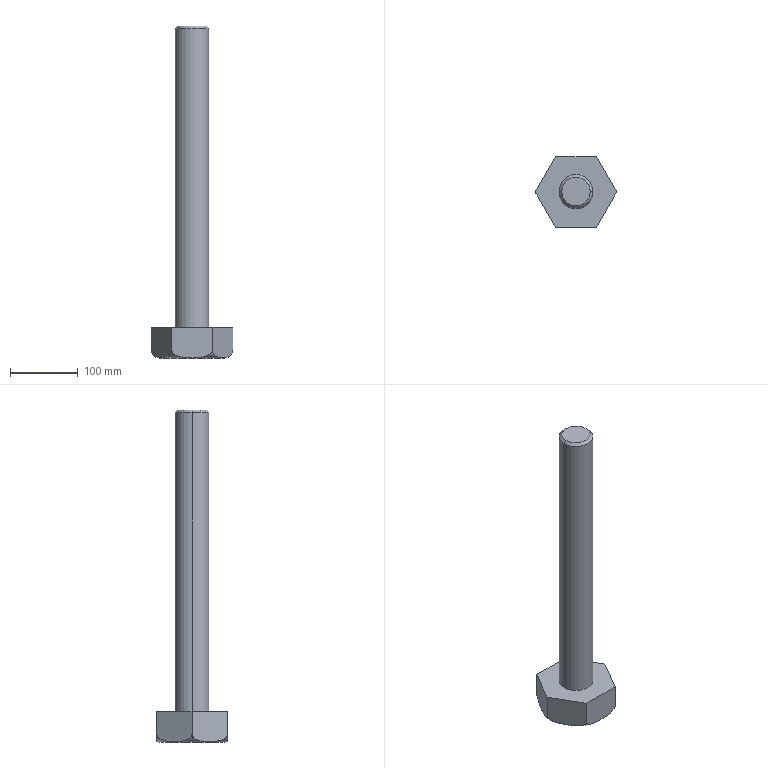Part | SolidWorks | features Chamfer 1, Extrusion 1, ICE 1, RevCut 1 | 1 solid | 15 faces | box 120.089 x 104 x 490 mm | volume 1291940 mm3 | plane 9 | cone 2 | cylinder 2 | torus 2 | commonest cylinder face diameters 50 x2
STEP:
#1=CARTESIAN_POINT('',(21.,0.,490.));
#2=VERTEX_POINT('',#1);
#3=CARTESIAN_POINT('',(-21.,0.,490.));
#4=VERTEX_POINT('',#3);
#5=CARTESIAN_POINT('',(0.,0.,490.));
#6=DIRECTION('',(0.,0.,1.));
#7=DIRECTION('',(1.,0.,0.));
#8=AXIS2_PLACEMENT_3D('',#5,#6,#7);
#9=CIRCLE('',#8,21.);
#10=EDGE_CURVE('',#2,#4,#9,.T.);
#11=ORIENTED_EDGE('',*,*,#10,.F.);
#12=CARTESIAN_POINT('',(25.,0.,486.));
#13=VERTEX_POINT('',#12);
#14=CARTESIAN_POINT('',(21.,0.,490.));
#15=DIRECTION('',(0.7071,0.,-0.7071));
#16=VECTOR('',#15,1000.);
#17=LINE('',#14,#16);
#18=EDGE_CURVE('',#2,#13,#17,.T.);
#19=ORIENTED_EDGE('',*,*,#18,.T.);
#20=CARTESIAN_POINT('',(-25.,0.,486.));
#21=VERTEX_POINT('',#20);
#22=CARTESIAN_POINT('',(0.,0.,486.));
#23=DIRECTION('',(0.,0.,-1.));
#24=DIRECTION('',(1.,0.,0.));
#25=AXIS2_PLACEMENT_3D('',#22,#23,#24);
#26=CIRCLE('',#25,25.);
#27=EDGE_CURVE('',#21,#13,#26,.T.);
#28=ORIENTED_EDGE('',*,*,#27,.F.);
#29=CARTESIAN_POINT('',(-21.,0.,490.));
#30=DIRECTION('',(-0.7071,0.,-0.7071));
#31=VECTOR('',#30,1000.);
#32=LINE('',#29,#31);
#33=EDGE_CURVE('',#4,#21,#32,.T.);
#34=ORIENTED_EDGE('',*,*,#33,.F.);
#35=EDGE_LOOP('',(#11,#19,#28,#34));
#36=FACE_OUTER_BOUND('',#35,.T.);
#37=CARTESIAN_POINT('',(0.,0.,490.));
#38=DIRECTION('',(0.,0.,-1.));
#39=DIRECTION('',(-1.,0.,0.));
#40=AXIS2_PLACEMENT_3D('',#37,#38,#39);
#41=CONICAL_SURFACE('',#40,21.,0.7854);
#42=ADVANCED_FACE('',(#36),#41,.T.);
#43=ORIENTED_EDGE('',*,*,#27,.T.);
#44=CARTESIAN_POINT('',(25.,0.,45.));
#45=VERTEX_POINT('',#44);
#46=CARTESIAN_POINT('',(25.,0.,490.));
#47=DIRECTION('',(0.,0.,-1.));
#48=VECTOR('',#47,1000.);
#49=LINE('',#46,#48);
#50=EDGE_CURVE('',#13,#45,#49,.T.);
#51=ORIENTED_EDGE('',*,*,#50,.T.);
#52=CARTESIAN_POINT('',(-25.,0.,45.));
#53=VERTEX_POINT('',#52);
#54=CARTESIAN_POINT('',(0.,0.,45.));
#55=DIRECTION('',(0.,0.,1.));
#56=DIRECTION('',(1.,0.,0.));
#57=AXIS2_PLACEMENT_3D('',#54,#55,#56);
#58=CIRCLE('',#57,25.);
#59=EDGE_CURVE('',#45,#53,#58,.T.);
#60=ORIENTED_EDGE('',*,*,#59,.T.);
#61=CARTESIAN_POINT('',(-25.,0.,490.));
#62=DIRECTION('',(0.,0.,-1.));
#63=VECTOR('',#62,1000.);
#64=LINE('',#61,#63);
#65=EDGE_CURVE('',#21,#53,#64,.T.);
#66=ORIENTED_EDGE('',*,*,#65,.F.);
#67=EDGE_LOOP('',(#43,#51,#60,#66));
#68=FACE_OUTER_BOUND('',#67,.T.);
#69=CARTESIAN_POINT('',(0.,0.,490.));
#70=DIRECTION('',(0.,0.,-1.));
#71=DIRECTION('',(-1.,0.,0.));
#72=AXIS2_PLACEMENT_3D('',#69,#70,#71);
#73=CYLINDRICAL_SURFACE('',#72,25.);
#74=ADVANCED_FACE('',(#68),#73,.T.);
#75=CARTESIAN_POINT('',(60.044,0.,12.));
#76=VERTEX_POINT('',#75);
#77=CARTESIAN_POINT('',(30.022,52.,12.));
#78=VERTEX_POINT('',#77);
#79=CARTESIAN_POINT('',(60.044,0.,12.));
#80=CARTESIAN_POINT('',(60.044,0.,11.26));
#81=CARTESIAN_POINT('',(59.977,0.1174,10.543));
#82=CARTESIAN_POINT('',(59.786,0.4482,9.504));
#83=CARTESIAN_POINT('',(59.709,0.5818,9.172));
#84=CARTESIAN_POINT('',(59.531,0.8892,8.533));
#85=CARTESIAN_POINT('',(59.43,1.064,8.225));
#86=CARTESIAN_POINT('',(59.1,1.636,7.342));
#87=CARTESIAN_POINT('',(58.847,2.074,6.819));
#88=CARTESIAN_POINT('',(58.296,3.028,5.867));
#89=CARTESIAN_POINT('',(57.996,3.549,5.437));
#90=CARTESIAN_POINT('',(57.376,4.621,4.673));
#91=CARTESIAN_POINT('',(57.056,5.177,4.336));
#92=CARTESIAN_POINT('',(56.398,6.316,3.728));
#93=CARTESIAN_POINT('',(56.061,6.9,3.458));
#94=CARTESIAN_POINT('',(55.373,8.092,2.971));
#95=CARTESIAN_POINT('',(55.024,8.695,2.757));
#96=CARTESIAN_POINT('',(54.326,9.905,2.375));
#97=CARTESIAN_POINT('',(53.975,10.513,2.207));
#98=CARTESIAN_POINT('',(52.919,12.342,1.759));
#99=CARTESIAN_POINT('',(52.209,13.571,1.533));
#100=CARTESIAN_POINT('',(50.783,16.041,1.175));
#101=CARTESIAN_POINT('',(50.066,17.282,1.044));
#102=CARTESIAN_POINT('',(48.629,19.773,0.8452));
#103=CARTESIAN_POINT('',(47.907,21.022,0.778));
#104=CARTESIAN_POINT('',(46.462,23.525,0.6906));
#105=CARTESIAN_POINT('',(45.74,24.776,0.6704));
#106=CARTESIAN_POINT('',(44.296,27.278,0.671));
#107=CARTESIAN_POINT('',(43.573,28.529,0.6918));
#108=CARTESIAN_POINT('',(42.129,31.03,0.7805));
#109=CARTESIAN_POINT('',(41.407,32.281,0.8485));
#110=CARTESIAN_POINT('',(39.966,34.777,1.05));
#111=CARTESIAN_POINT('',(39.248,36.021,1.183));
#112=CARTESIAN_POINT('',(37.817,38.5,1.545));
#113=CARTESIAN_POINT('',(37.104,39.735,1.775));
#114=CARTESIAN_POINT('',(35.687,42.188,2.382));
#115=CARTESIAN_POINT('',(34.991,43.394,2.757));
#116=CARTESIAN_POINT('',(33.974,45.156,3.483));
#117=CARTESIAN_POINT('',(33.639,45.735,3.753));
#118=CARTESIAN_POINT('',(32.982,46.873,4.365));
#119=CARTESIAN_POINT('',(32.66,47.431,4.707));
#120=CARTESIAN_POINT('',(32.046,48.494,5.471));
#121=CARTESIAN_POINT('',(31.753,49.002,5.893));
#122=CARTESIAN_POINT('',(31.203,49.954,6.85));
#123=CARTESIAN_POINT('',(30.953,50.387,7.374));
#124=CARTESIAN_POINT('',(30.63,50.948,8.245));
#125=CARTESIAN_POINT('',(30.53,51.12,8.551));
#126=CARTESIAN_POINT('',(30.354,51.426,9.19));
#127=CARTESIAN_POINT('',(30.278,51.557,9.519));
#128=CARTESIAN_POINT('',(30.154,51.772,10.198));
#129=CARTESIAN_POINT('',(30.105,51.857,10.55));
#130=CARTESIAN_POINT('',(30.039,51.971,11.27));
#131=CARTESIAN_POINT('',(30.022,52.,11.633));
#132=CARTESIAN_POINT('',(30.022,52.,12.));
#133=B_SPLINE_CURVE_WITH_KNOTS('',3,(#79,#80,#81,#82,#83,#84,#85,#86,#87,#88,#89,#90,#91,#92,#93,#94,#95,#96,#97,#98,#99,#100,#101,#102,#103,#104,#105,#106,#107,#108,#109,#110,#111,#112,#113,#114,#115,#116,#117,#118,#119,#120,#121,#122,#123,#124,#125,#126,#127,#128,#129,#130,#131,#132),.UNSPECIFIED.,.F.,.F.,(4,2,2,2,2,2,2,2,2,2,2,2,2,2,2,2,2,2,2,2,2,2,2,2,2,2,4),(0.000000197,0.002185,0.003278,0.00437,0.006555,0.00874,0.01093,0.01311,0.0153,0.01748,0.02185,0.02622,0.03059,0.03496,0.03933,0.0437,0.04807,0.05244,0.05681,0.059,0.06118,0.06337,0.06555,0.06664,0.06774,0.06883,0.06992),.UNSPECIFIED.);
#134=EDGE_CURVE('',#76,#78,#133,.T.);
#135=ORIENTED_EDGE('',*,*,#134,.F.);
#136=CARTESIAN_POINT('',(48.044,0.,0.));
#137=VERTEX_POINT('',#136);
#138=CARTESIAN_POINT('',(48.044,0.,12.));
#139=DIRECTION('',(0.,1.,0.));
#140=DIRECTION('',(-1.,0.,0.));
#141=AXIS2_PLACEMENT_3D('',#138,#139,#140);
#142=CIRCLE('',#141,12.);
#143=EDGE_CURVE('',#76,#137,#142,.T.);
#144=ORIENTED_EDGE('',*,*,#143,.T.);
#145=CARTESIAN_POINT('',(-48.044,0.,0.));
#146=VERTEX_POINT('',#145);
#147=CARTESIAN_POINT('',(0.,0.,0.));
#148=DIRECTION('',(0.,0.,-1.));
#149=DIRECTION('',(-1.,0.,0.));
#150=AXIS2_PLACEMENT_3D('',#147,#148,#149);
#151=CIRCLE('',#150,48.044);
#152=EDGE_CURVE('',#146,#137,#151,.T.);
#153=ORIENTED_EDGE('',*,*,#152,.F.);
#154=CARTESIAN_POINT('',(-60.044,0.,12.));
#155=VERTEX_POINT('',#154);
#156=CARTESIAN_POINT('',(-48.044,0.,12.));
#157=DIRECTION('',(0.,-1.,0.));
#158=DIRECTION('',(0.,0.,-1.));
#159=AXIS2_PLACEMENT_3D('',#156,#157,#158);
#160=CIRCLE('',#159,12.);
#161=EDGE_CURVE('',#155,#146,#160,.T.);
#162=ORIENTED_EDGE('',*,*,#161,.F.);
#163=CARTESIAN_POINT('',(-30.022,52.,12.));
#164=VERTEX_POINT('',#163);
#165=CARTESIAN_POINT('',(-30.022,52.,12.));
#166=CARTESIAN_POINT('',(-30.022,52.,11.26));
#167=CARTESIAN_POINT('',(-30.09,51.883,10.543));
#168=CARTESIAN_POINT('',(-30.281,51.552,9.504));
#169=CARTESIAN_POINT('',(-30.358,51.418,9.172));
#170=CARTESIAN_POINT('',(-30.536,51.111,8.533));
#171=CARTESIAN_POINT('',(-30.636,50.936,8.225));
#172=CARTESIAN_POINT('',(-30.967,50.364,7.342));
#173=CARTESIAN_POINT('',(-31.22,49.926,6.819));
#174=CARTESIAN_POINT('',(-31.77,48.972,5.867));
#175=CARTESIAN_POINT('',(-32.071,48.451,5.437));
#176=CARTESIAN_POINT('',(-32.69,47.379,4.673));
#177=CARTESIAN_POINT('',(-33.011,46.823,4.336));
#178=CARTESIAN_POINT('',(-33.669,45.684,3.728));
#179=CARTESIAN_POINT('',(-34.006,45.1,3.458));
#180=CARTESIAN_POINT('',(-34.694,43.908,2.971));
#181=CARTESIAN_POINT('',(-35.043,43.305,2.757));
#182=CARTESIAN_POINT('',(-35.741,42.095,2.375));
#183=CARTESIAN_POINT('',(-36.092,41.487,2.207));
#184=CARTESIAN_POINT('',(-37.148,39.658,1.759));
#185=CARTESIAN_POINT('',(-37.858,38.429,1.533));
#186=CARTESIAN_POINT('',(-39.284,35.959,1.175));
#187=CARTESIAN_POINT('',(-40.,34.718,1.044));
#188=CARTESIAN_POINT('',(-41.438,32.227,0.8452));
#189=CARTESIAN_POINT('',(-42.159,30.978,0.778));
#190=CARTESIAN_POINT('',(-43.604,28.475,0.6906));
#191=CARTESIAN_POINT('',(-44.327,27.224,0.6704));
#192=CARTESIAN_POINT('',(-45.771,24.722,0.671));
#193=CARTESIAN_POINT('',(-46.493,23.471,0.6918));
#194=CARTESIAN_POINT('',(-47.937,20.97,0.7805));
#195=CARTESIAN_POINT('',(-48.66,19.719,0.8485));
#196=CARTESIAN_POINT('',(-50.101,17.223,1.05));
#197=CARTESIAN_POINT('',(-50.819,15.979,1.183));
#198=CARTESIAN_POINT('',(-52.25,13.5,1.545));
#199=CARTESIAN_POINT('',(-52.963,12.265,1.775));
#200=CARTESIAN_POINT('',(-54.38,9.812,2.382));
#201=CARTESIAN_POINT('',(-55.076,8.606,2.757));
#202=CARTESIAN_POINT('',(-56.093,6.844,3.483));
#203=CARTESIAN_POINT('',(-56.427,6.265,3.753));
#204=CARTESIAN_POINT('',(-57.084,5.127,4.365));
#205=CARTESIAN_POINT('',(-57.406,4.569,4.707));
#206=CARTESIAN_POINT('',(-58.02,3.506,5.471));
#207=CARTESIAN_POINT('',(-58.314,2.998,5.893));
#208=CARTESIAN_POINT('',(-58.863,2.046,6.85));
#209=CARTESIAN_POINT('',(-59.113,1.613,7.374));
#210=CARTESIAN_POINT('',(-59.437,1.052,8.245));
#211=CARTESIAN_POINT('',(-59.537,0.8795,8.551));
#212=CARTESIAN_POINT('',(-59.713,0.5743,9.19));
#213=CARTESIAN_POINT('',(-59.789,0.4431,9.519));
#214=CARTESIAN_POINT('',(-59.913,0.2276,10.198));
#215=CARTESIAN_POINT('',(-59.962,0.1431,10.55));
#216=CARTESIAN_POINT('',(-60.028,0.02903,11.27));
#217=CARTESIAN_POINT('',(-60.044,0.,11.633));
#218=CARTESIAN_POINT('',(-60.044,0.,12.));
#219=B_SPLINE_CURVE_WITH_KNOTS('',3,(#165,#166,#167,#168,#169,#170,#171,#172,#173,#174,#175,#176,#177,#178,#179,#180,#181,#182,#183,#184,#185,#186,#187,#188,#189,#190,#191,#192,#193,#194,#195,#196,#197,#198,#199,#200,#201,#202,#203,#204,#205,#206,#207,#208,#209,#210,#211,#212,#213,#214,#215,#216,#217,#218),.UNSPECIFIED.,.F.,.F.,(4,2,2,2,2,2,2,2,2,2,2,2,2,2,2,2,2,2,2,2,2,2,2,2,2,2,4),(0.000000197,0.002185,0.003278,0.00437,0.006555,0.00874,0.01093,0.01311,0.0153,0.01748,0.02185,0.02622,0.03059,0.03496,0.03933,0.0437,0.04807,0.05244,0.05681,0.059,0.06118,0.06337,0.06555,0.06664,0.06774,0.06883,0.06992),.UNSPECIFIED.);
#220=EDGE_CURVE('',#164,#155,#219,.T.);
#221=ORIENTED_EDGE('',*,*,#220,.F.);
#222=CARTESIAN_POINT('',(30.022,52.,12.));
#223=CARTESIAN_POINT('',(30.022,52.,11.638));
#224=CARTESIAN_POINT('',(29.99,52.,11.278));
#225=CARTESIAN_POINT('',(29.892,52.,10.738));
#226=CARTESIAN_POINT('',(29.851,52.,10.558));
#227=CARTESIAN_POINT('',(29.754,52.,10.205));
#228=CARTESIAN_POINT('',(29.698,52.,10.031));
#229=CARTESIAN_POINT('',(29.511,52.,9.519));
#230=CARTESIAN_POINT('',(29.358,52.,9.188));
#231=CARTESIAN_POINT('',(29.003,52.,8.545));
#232=CARTESIAN_POINT('',(28.803,52.,8.239));
#233=CARTESIAN_POINT('',(28.37,52.,7.657));
#234=CARTESIAN_POINT('',(28.136,52.,7.381));
#235=CARTESIAN_POINT('',(27.638,52.,6.852));
#236=CARTESIAN_POINT('',(27.373,52.,6.6));
#237=CARTESIAN_POINT('',(26.545,52.,5.881));
#238=CARTESIAN_POINT('',(25.957,52.,5.459));
#239=CARTESIAN_POINT('',(24.73,52.,4.698));
#240=CARTESIAN_POINT('',(24.09,52.,4.358));
#241=CARTESIAN_POINT('',(22.769,52.,3.745));
#242=CARTESIAN_POINT('',(22.095,52.,3.474));
#243=CARTESIAN_POINT('',(20.055,52.,2.748));
#244=CARTESIAN_POINT('',(18.664,52.,2.376));
#245=CARTESIAN_POINT('',(15.845,52.,1.772));
#246=CARTESIAN_POINT('',(14.413,52.,1.542));
#247=CARTESIAN_POINT('',(11.542,52.,1.179));
#248=CARTESIAN_POINT('',(10.104,52.,1.047));
#249=CARTESIAN_POINT('',(7.223,52.,0.8469));
#250=CARTESIAN_POINT('',(5.78,52.,0.7794));
#251=CARTESIAN_POINT('',(2.893,52.,0.6913));
#252=CARTESIAN_POINT('',(1.447,52.,0.6707));
#253=CARTESIAN_POINT('',(-1.446,52.,0.6707));
#254=CARTESIAN_POINT('',(-2.887,52.,0.6912));
#255=CARTESIAN_POINT('',(-5.77,52.,0.779));
#256=CARTESIAN_POINT('',(-7.209,52.,0.8462));
#257=CARTESIAN_POINT('',(-10.083,52.,1.045));
#258=CARTESIAN_POINT('',(-11.517,52.,1.177));
#259=CARTESIAN_POINT('',(-14.376,52.,1.537));
#260=CARTESIAN_POINT('',(-15.802,52.,1.764));
#261=CARTESIAN_POINT('',(-17.931,52.,2.218));
#262=CARTESIAN_POINT('',(-18.638,52.,2.388));
#263=CARTESIAN_POINT('',(-20.03,52.,2.771));
#264=CARTESIAN_POINT('',(-20.718,52.,2.984));
#265=CARTESIAN_POINT('',(-22.071,52.,3.465));
#266=CARTESIAN_POINT('',(-22.737,52.,3.732));
#267=CARTESIAN_POINT('',(-24.042,52.,4.334));
#268=CARTESIAN_POINT('',(-24.68,52.,4.67));
#269=CARTESIAN_POINT('',(-25.61,52.,5.243));
#270=CARTESIAN_POINT('',(-25.917,52.,5.447));
#271=CARTESIAN_POINT('',(-26.511,52.,5.877));
#272=CARTESIAN_POINT('',(-26.799,52.,6.103));
#273=CARTESIAN_POINT('',(-27.35,52.,6.579));
#274=CARTESIAN_POINT('',(-27.615,52.,6.829));
#275=CARTESIAN_POINT('',(-28.117,52.,7.359));
#276=CARTESIAN_POINT('',(-28.355,52.,7.639));
#277=CARTESIAN_POINT('',(-29.018,52.,8.525));
#278=CARTESIAN_POINT('',(-29.379,52.,9.16));
#279=CARTESIAN_POINT('',(-29.761,52.,10.2));
#280=CARTESIAN_POINT('',(-29.858,52.,10.555));
#281=CARTESIAN_POINT('',(-29.989,52.,11.27));
#282=CARTESIAN_POINT('',(-30.022,52.,11.633));
#283=CARTESIAN_POINT('',(-30.022,52.,12.));
#284=B_SPLINE_CURVE_WITH_KNOTS('',3,(#222,#223,#224,#225,#226,#227,#228,#229,#230,#231,#232,#233,#234,#235,#236,#237,#238,#239,#240,#241,#242,#243,#244,#245,#246,#247,#248,#249,#250,#251,#252,#253,#254,#255,#256,#257,#258,#259,#260,#261,#262,#263,#264,#265,#266,#267,#268,#269,#270,#271,#272,#273,#274,#275,#276,#277,#278,#279,#280,#281,#282,#283),.UNSPECIFIED.,.F.,.F.,(4,2,2,2,2,2,2,2,2,2,2,2,2,2,2,2,2,2,2,2,2,2,2,2,2,2,2,2,2,2,4),(0.1036,0.1047,0.1052,0.1058,0.1068,0.1079,0.109,0.1101,0.1122,0.1144,0.1166,0.1209,0.1252,0.1295,0.1338,0.1382,0.1425,0.1468,0.1511,0.1554,0.1576,0.1598,0.1619,0.1641,0.1652,0.1662,0.1673,0.1684,0.1706,0.1716,0.1727),.UNSPECIFIED.);
#285=EDGE_CURVE('',#78,#164,#284,.T.);
#286=ORIENTED_EDGE('',*,*,#285,.F.);
#287=EDGE_LOOP('',(#135,#144,#153,#162,#221,#286));
#288=FACE_OUTER_BOUND('',#287,.T.);
#289=CARTESIAN_POINT('',(0.,0.,12.));
#290=DIRECTION('',(0.,0.,-1.));
#291=DIRECTION('',(-1.,0.,0.));
#292=AXIS2_PLACEMENT_3D('',#289,#290,#291);
#293=TOROIDAL_SURFACE('',#292,48.044,12.);
#294=ADVANCED_FACE('',(#288),#293,.T.);
#295=CARTESIAN_POINT('',(-30.022,-52.,45.));
#296=VERTEX_POINT('',#295);
#297=CARTESIAN_POINT('',(30.022,-52.,45.));
#298=VERTEX_POINT('',#297);
#299=CARTESIAN_POINT('',(-30.022,-52.,45.));
#300=DIRECTION('',(1.,0.,0.));
#301=VECTOR('',#300,1000.);
#302=LINE('',#299,#301);
#303=EDGE_CURVE('',#296,#298,#302,.T.);
#304=ORIENTED_EDGE('',*,*,#303,.T.);
#305=CARTESIAN_POINT('',(60.044,0.,45.));
#306=VERTEX_POINT('',#305);
#307=CARTESIAN_POINT('',(30.022,-52.,45.));
#308=DIRECTION('',(0.5,0.866,0.));
#309=VECTOR('',#308,1000.);
#310=LINE('',#307,#309);
#311=EDGE_CURVE('',#298,#306,#310,.T.);
#312=ORIENTED_EDGE('',*,*,#311,.T.);
#313=CARTESIAN_POINT('',(30.022,52.,45.));
#314=VERTEX_POINT('',#313);
#315=CARTESIAN_POINT('',(60.044,0.,45.));
#316=DIRECTION('',(-0.5,0.866,0.));
#317=VECTOR('',#316,1000.);
#318=LINE('',#315,#317);
#319=EDGE_CURVE('',#306,#314,#318,.T.);
#320=ORIENTED_EDGE('',*,*,#319,.T.);
#321=CARTESIAN_POINT('',(-30.022,52.,45.));
#322=VERTEX_POINT('',#321);
#323=CARTESIAN_POINT('',(30.022,52.,45.));
#324=DIRECTION('',(-1.,0.,0.));
#325=VECTOR('',#324,1000.);
#326=LINE('',#323,#325);
#327=EDGE_CURVE('',#314,#322,#326,.T.);
#328=ORIENTED_EDGE('',*,*,#327,.T.);
#329=CARTESIAN_POINT('',(-60.044,0.,45.));
#330=VERTEX_POINT('',#329);
#331=CARTESIAN_POINT('',(-30.022,52.,45.));
#332=DIRECTION('',(-0.5,-0.866,0.));
#333=VECTOR('',#332,1000.);
#334=LINE('',#331,#333);
#335=EDGE_CURVE('',#322,#330,#334,.T.);
#336=ORIENTED_EDGE('',*,*,#335,.T.);
#337=CARTESIAN_POINT('',(-60.044,0.,45.));
#338=DIRECTION('',(0.5,-0.866,0.));
#339=VECTOR('',#338,1000.);
#340=LINE('',#337,#339);
#341=EDGE_CURVE('',#330,#296,#340,.T.);
#342=ORIENTED_EDGE('',*,*,#341,.T.);
#343=EDGE_LOOP('',(#304,#312,#320,#328,#336,#342));
#344=FACE_OUTER_BOUND('',#343,.T.);
#345=CARTESIAN_POINT('',(0.,0.,45.));
#346=DIRECTION('',(0.,0.,1.));
#347=DIRECTION('',(1.,0.,0.));
#348=AXIS2_PLACEMENT_3D('',#345,#346,#347);
#349=CIRCLE('',#348,25.);
#350=EDGE_CURVE('',#53,#45,#349,.T.);
#351=ORIENTED_EDGE('',*,*,#350,.F.);
#352=ORIENTED_EDGE('',*,*,#59,.F.);
#353=EDGE_LOOP('',(#351,#352));
#354=FACE_BOUND('',#353,.T.);
#355=CARTESIAN_POINT('',(0.,0.,45.));
#356=DIRECTION('',(0.,0.,1.));
#357=DIRECTION('',(1.,0.,0.));
#358=AXIS2_PLACEMENT_3D('',#355,#356,#357);
#359=PLANE('',#358);
#360=ADVANCED_FACE('',(#344,#354),#359,.T.);
#361=CARTESIAN_POINT('',(-30.022,-52.,12.));
#362=VERTEX_POINT('',#361);
#363=CARTESIAN_POINT('',(-30.022,-52.,45.));
#364=DIRECTION('',(0.,0.,-1.));
#365=VECTOR('',#364,1000.);
#366=LINE('',#363,#365);
#367=EDGE_CURVE('',#296,#362,#366,.T.);
#368=ORIENTED_EDGE('',*,*,#367,.T.);
#369=CARTESIAN_POINT('',(30.022,-52.,12.));
#370=VERTEX_POINT('',#369);
#371=CARTESIAN_POINT('',(-30.022,-52.,12.));
#372=CARTESIAN_POINT('',(-30.022,-52.,11.638));
#373=CARTESIAN_POINT('',(-29.99,-52.,11.278));
#374=CARTESIAN_POINT('',(-29.892,-52.,10.738));
#375=CARTESIAN_POINT('',(-29.851,-52.,10.558));
#376=CARTESIAN_POINT('',(-29.754,-52.,10.205));
#377=CARTESIAN_POINT('',(-29.698,-52.,10.031));
#378=CARTESIAN_POINT('',(-29.511,-52.,9.519));
#379=CARTESIAN_POINT('',(-29.358,-52.,9.188));
#380=CARTESIAN_POINT('',(-29.003,-52.,8.545));
#381=CARTESIAN_POINT('',(-28.803,-52.,8.239));
#382=CARTESIAN_POINT('',(-28.37,-52.,7.657));
#383=CARTESIAN_POINT('',(-28.136,-52.,7.381));
#384=CARTESIAN_POINT('',(-27.638,-52.,6.852));
#385=CARTESIAN_POINT('',(-27.373,-52.,6.6));
#386=CARTESIAN_POINT('',(-26.545,-52.,5.881));
#387=CARTESIAN_POINT('',(-25.957,-52.,5.459));
#388=CARTESIAN_POINT('',(-24.73,-52.,4.698));
#389=CARTESIAN_POINT('',(-24.09,-52.,4.358));
#390=CARTESIAN_POINT('',(-22.769,-52.,3.745));
#391=CARTESIAN_POINT('',(-22.095,-52.,3.474));
#392=CARTESIAN_POINT('',(-20.055,-52.,2.748));
#393=CARTESIAN_POINT('',(-18.664,-52.,2.376));
#394=CARTESIAN_POINT('',(-15.845,-52.,1.772));
#395=CARTESIAN_POINT('',(-14.413,-52.,1.542));
#396=CARTESIAN_POINT('',(-11.542,-52.,1.179));
#397=CARTESIAN_POINT('',(-10.104,-52.,1.047));
#398=CARTESIAN_POINT('',(-7.223,-52.,0.8469));
#399=CARTESIAN_POINT('',(-5.78,-52.,0.7794));
#400=CARTESIAN_POINT('',(-2.893,-52.,0.6913));
#401=CARTESIAN_POINT('',(-1.447,-52.,0.6707));
#402=CARTESIAN_POINT('',(1.446,-52.,0.6707));
#403=CARTESIAN_POINT('',(2.887,-52.,0.6912));
#404=CARTESIAN_POINT('',(5.77,-52.,0.779));
#405=CARTESIAN_POINT('',(7.209,-52.,0.8462));
#406=CARTESIAN_POINT('',(10.083,-52.,1.045));
#407=CARTESIAN_POINT('',(11.517,-52.,1.177));
#408=CARTESIAN_POINT('',(14.376,-52.,1.537));
#409=CARTESIAN_POINT('',(15.802,-52.,1.764));
#410=CARTESIAN_POINT('',(17.931,-52.,2.218));
#411=CARTESIAN_POINT('',(18.638,-52.,2.388));
#412=CARTESIAN_POINT('',(20.03,-52.,2.771));
#413=CARTESIAN_POINT('',(20.718,-52.,2.984));
#414=CARTESIAN_POINT('',(22.071,-52.,3.465));
#415=CARTESIAN_POINT('',(22.737,-52.,3.732));
#416=CARTESIAN_POINT('',(24.042,-52.,4.334));
#417=CARTESIAN_POINT('',(24.68,-52.,4.67));
#418=CARTESIAN_POINT('',(25.61,-52.,5.243));
#419=CARTESIAN_POINT('',(25.917,-52.,5.447));
#420=CARTESIAN_POINT('',(26.511,-52.,5.877));
#421=CARTESIAN_POINT('',(26.799,-52.,6.103));
#422=CARTESIAN_POINT('',(27.35,-52.,6.579));
#423=CARTESIAN_POINT('',(27.615,-52.,6.829));
#424=CARTESIAN_POINT('',(28.117,-52.,7.359));
#425=CARTESIAN_POINT('',(28.355,-52.,7.639));
#426=CARTESIAN_POINT('',(29.018,-52.,8.525));
#427=CARTESIAN_POINT('',(29.379,-52.,9.16));
#428=CARTESIAN_POINT('',(29.761,-52.,10.2));
#429=CARTESIAN_POINT('',(29.858,-52.,10.555));
#430=CARTESIAN_POINT('',(29.989,-52.,11.27));
#431=CARTESIAN_POINT('',(30.022,-52.,11.633));
#432=CARTESIAN_POINT('',(30.022,-52.,12.));
#433=B_SPLINE_CURVE_WITH_KNOTS('',3,(#371,#372,#373,#374,#375,#376,#377,#378,#379,#380,#381,#382,#383,#384,#385,#386,#387,#388,#389,#390,#391,#392,#393,#394,#395,#396,#397,#398,#399,#400,#401,#402,#403,#404,#405,#406,#407,#408,#409,#410,#411,#412,#413,#414,#415,#416,#417,#418,#419,#420,#421,#422,#423,#424,#425,#426,#427,#428,#429,#430,#431,#432),.UNSPECIFIED.,.F.,.F.,(4,2,2,2,2,2,2,2,2,2,2,2,2,2,2,2,2,2,2,2,2,2,2,2,2,2,2,2,2,2,4),(0.1036,0.1047,0.1052,0.1058,0.1068,0.1079,0.109,0.1101,0.1122,0.1144,0.1166,0.1209,0.1252,0.1295,0.1338,0.1382,0.1425,0.1468,0.1511,0.1554,0.1576,0.1598,0.1619,0.1641,0.1652,0.1662,0.1673,0.1684,0.1706,0.1716,0.1727),.UNSPECIFIED.);
#434=EDGE_CURVE('',#362,#370,#433,.T.);
#435=ORIENTED_EDGE('',*,*,#434,.T.);
#436=CARTESIAN_POINT('',(30.022,-52.,45.));
#437=DIRECTION('',(0.,0.,-1.));
#438=VECTOR('',#437,1000.);
#439=LINE('',#436,#438);
#440=EDGE_CURVE('',#298,#370,#439,.T.);
#441=ORIENTED_EDGE('',*,*,#440,.F.);
#442=ORIENTED_EDGE('',*,*,#303,.F.);
#443=EDGE_LOOP('',(#368,#435,#441,#442));
#444=FACE_OUTER_BOUND('',#443,.T.);
#445=CARTESIAN_POINT('',(-30.022,-52.,45.));
#446=DIRECTION('',(0.,1.,0.));
#447=DIRECTION('',(-1.,0.,0.));
#448=AXIS2_PLACEMENT_3D('',#445,#446,#447);
#449=PLANE('',#448);
#450=ADVANCED_FACE('',(#444),#449,.F.);
#451=ORIENTED_EDGE('',*,*,#440,.T.);
#452=CARTESIAN_POINT('',(30.022,-52.,12.));
#453=CARTESIAN_POINT('',(30.022,-52.,11.26));
#454=CARTESIAN_POINT('',(30.09,-51.883,10.543));
#455=CARTESIAN_POINT('',(30.281,-51.552,9.504));
#456=CARTESIAN_POINT('',(30.358,-51.418,9.172));
#457=CARTESIAN_POINT('',(30.536,-51.111,8.533));
#458=CARTESIAN_POINT('',(30.636,-50.936,8.225));
#459=CARTESIAN_POINT('',(30.967,-50.364,7.342));
#460=CARTESIAN_POINT('',(31.22,-49.926,6.819));
#461=CARTESIAN_POINT('',(31.77,-48.972,5.867));
#462=CARTESIAN_POINT('',(32.071,-48.451,5.437));
#463=CARTESIAN_POINT('',(32.69,-47.379,4.673));
#464=CARTESIAN_POINT('',(33.011,-46.823,4.336));
#465=CARTESIAN_POINT('',(33.669,-45.684,3.728));
#466=CARTESIAN_POINT('',(34.006,-45.1,3.458));
#467=CARTESIAN_POINT('',(34.694,-43.908,2.971));
#468=CARTESIAN_POINT('',(35.043,-43.305,2.757));
#469=CARTESIAN_POINT('',(35.741,-42.095,2.375));
#470=CARTESIAN_POINT('',(36.092,-41.487,2.207));
#471=CARTESIAN_POINT('',(37.148,-39.658,1.759));
#472=CARTESIAN_POINT('',(37.858,-38.429,1.533));
#473=CARTESIAN_POINT('',(39.284,-35.959,1.175));
#474=CARTESIAN_POINT('',(40.,-34.718,1.044));
#475=CARTESIAN_POINT('',(41.438,-32.227,0.8452));
#476=CARTESIAN_POINT('',(42.159,-30.978,0.778));
#477=CARTESIAN_POINT('',(43.604,-28.475,0.6906));
#478=CARTESIAN_POINT('',(44.327,-27.224,0.6704));
#479=CARTESIAN_POINT('',(45.771,-24.722,0.671));
#480=CARTESIAN_POINT('',(46.493,-23.471,0.6918));
#481=CARTESIAN_POINT('',(47.937,-20.97,0.7805));
#482=CARTESIAN_POINT('',(48.66,-19.719,0.8485));
#483=CARTESIAN_POINT('',(50.101,-17.223,1.05));
#484=CARTESIAN_POINT('',(50.819,-15.979,1.183));
#485=CARTESIAN_POINT('',(52.25,-13.5,1.545));
#486=CARTESIAN_POINT('',(52.963,-12.265,1.775));
#487=CARTESIAN_POINT('',(54.38,-9.812,2.382));
#488=CARTESIAN_POINT('',(55.076,-8.606,2.757));
#489=CARTESIAN_POINT('',(56.093,-6.844,3.483));
#490=CARTESIAN_POINT('',(56.427,-6.265,3.753));
#491=CARTESIAN_POINT('',(57.084,-5.127,4.365));
#492=CARTESIAN_POINT('',(57.406,-4.569,4.707));
#493=CARTESIAN_POINT('',(58.02,-3.506,5.471));
#494=CARTESIAN_POINT('',(58.314,-2.998,5.893));
#495=CARTESIAN_POINT('',(58.863,-2.046,6.85));
#496=CARTESIAN_POINT('',(59.113,-1.613,7.374));
#497=CARTESIAN_POINT('',(59.437,-1.052,8.245));
#498=CARTESIAN_POINT('',(59.537,-0.8795,8.551));
#499=CARTESIAN_POINT('',(59.713,-0.5743,9.19));
#500=CARTESIAN_POINT('',(59.789,-0.4431,9.519));
#501=CARTESIAN_POINT('',(59.913,-0.2276,10.198));
#502=CARTESIAN_POINT('',(59.962,-0.1431,10.55));
#503=CARTESIAN_POINT('',(60.028,-0.02903,11.27));
#504=CARTESIAN_POINT('',(60.044,0.,11.633));
#505=CARTESIAN_POINT('',(60.044,0.,12.));
#506=B_SPLINE_CURVE_WITH_KNOTS('',3,(#452,#453,#454,#455,#456,#457,#458,#459,#460,#461,#462,#463,#464,#465,#466,#467,#468,#469,#470,#471,#472,#473,#474,#475,#476,#477,#478,#479,#480,#481,#482,#483,#484,#485,#486,#487,#488,#489,#490,#491,#492,#493,#494,#495,#496,#497,#498,#499,#500,#501,#502,#503,#504,#505),.UNSPECIFIED.,.F.,.F.,(4,2,2,2,2,2,2,2,2,2,2,2,2,2,2,2,2,2,2,2,2,2,2,2,2,2,4),(0.000000197,0.002185,0.003278,0.00437,0.006555,0.00874,0.01093,0.01311,0.0153,0.01748,0.02185,0.02622,0.03059,0.03496,0.03933,0.0437,0.04807,0.05244,0.05681,0.059,0.06118,0.06337,0.06555,0.06664,0.06774,0.06883,0.06992),.UNSPECIFIED.);
#507=EDGE_CURVE('',#370,#76,#506,.T.);
#508=ORIENTED_EDGE('',*,*,#507,.T.);
#509=CARTESIAN_POINT('',(60.044,0.,45.));
#510=DIRECTION('',(0.,0.,-1.));
#511=VECTOR('',#510,1000.);
#512=LINE('',#509,#511);
#513=EDGE_CURVE('',#306,#76,#512,.T.);
#514=ORIENTED_EDGE('',*,*,#513,.F.);
#515=ORIENTED_EDGE('',*,*,#311,.F.);
#516=EDGE_LOOP('',(#451,#508,#514,#515));
#517=FACE_OUTER_BOUND('',#516,.T.);
#518=CARTESIAN_POINT('',(30.022,-52.,45.));
#519=DIRECTION('',(-0.866,0.5,0.));
#520=DIRECTION('',(-0.5,-0.866,0.));
#521=AXIS2_PLACEMENT_3D('',#518,#519,#520);
#522=PLANE('',#521);
#523=ADVANCED_FACE('',(#517),#522,.F.);
#524=ORIENTED_EDGE('',*,*,#513,.T.);
#525=ORIENTED_EDGE('',*,*,#134,.T.);
#526=CARTESIAN_POINT('',(30.022,52.,45.));
#527=DIRECTION('',(0.,0.,-1.));
#528=VECTOR('',#527,1000.);
#529=LINE('',#526,#528);
#530=EDGE_CURVE('',#314,#78,#529,.T.);
#531=ORIENTED_EDGE('',*,*,#530,.F.);
#532=ORIENTED_EDGE('',*,*,#319,.F.);
#533=EDGE_LOOP('',(#524,#525,#531,#532));
#534=FACE_OUTER_BOUND('',#533,.T.);
#535=CARTESIAN_POINT('',(60.044,0.,45.));
#536=DIRECTION('',(-0.866,-0.5,0.));
#537=DIRECTION('',(0.5,-0.866,0.));
#538=AXIS2_PLACEMENT_3D('',#535,#536,#537);
#539=PLANE('',#538);
#540=ADVANCED_FACE('',(#534),#539,.F.);
#541=ORIENTED_EDGE('',*,*,#530,.T.);
#542=ORIENTED_EDGE('',*,*,#285,.T.);
#543=CARTESIAN_POINT('',(-30.022,52.,45.));
#544=DIRECTION('',(0.,0.,-1.));
#545=VECTOR('',#544,1000.);
#546=LINE('',#543,#545);
#547=EDGE_CURVE('',#322,#164,#546,.T.);
#548=ORIENTED_EDGE('',*,*,#547,.F.);
#549=ORIENTED_EDGE('',*,*,#327,.F.);
#550=EDGE_LOOP('',(#541,#542,#548,#549));
#551=FACE_OUTER_BOUND('',#550,.T.);
#552=CARTESIAN_POINT('',(30.022,52.,45.));
#553=DIRECTION('',(0.,-1.,0.));
#554=DIRECTION('',(1.,0.,0.));
#555=AXIS2_PLACEMENT_3D('',#552,#553,#554);
#556=PLANE('',#555);
#557=ADVANCED_FACE('',(#551),#556,.F.);
#558=ORIENTED_EDGE('',*,*,#547,.T.);
#559=ORIENTED_EDGE('',*,*,#220,.T.);
#560=CARTESIAN_POINT('',(-60.044,0.,45.));
#561=DIRECTION('',(0.,0.,-1.));
#562=VECTOR('',#561,1000.);
#563=LINE('',#560,#562);
#564=EDGE_CURVE('',#330,#155,#563,.T.);
#565=ORIENTED_EDGE('',*,*,#564,.F.);
#566=ORIENTED_EDGE('',*,*,#335,.F.);
#567=EDGE_LOOP('',(#558,#559,#565,#566));
#568=FACE_OUTER_BOUND('',#567,.T.);
#569=CARTESIAN_POINT('',(-30.022,52.,45.));
#570=DIRECTION('',(0.866,-0.5,0.));
#571=DIRECTION('',(0.5,0.866,0.));
#572=AXIS2_PLACEMENT_3D('',#569,#570,#571);
#573=PLANE('',#572);
#574=ADVANCED_FACE('',(#568),#573,.F.);
#575=ORIENTED_EDGE('',*,*,#564,.T.);
#576=CARTESIAN_POINT('',(-60.044,0.,12.));
#577=CARTESIAN_POINT('',(-60.044,0.,11.26));
#578=CARTESIAN_POINT('',(-59.977,-0.1174,10.543));
#579=CARTESIAN_POINT('',(-59.786,-0.4482,9.504));
#580=CARTESIAN_POINT('',(-59.709,-0.5818,9.172));
#581=CARTESIAN_POINT('',(-59.531,-0.8892,8.533));
#582=CARTESIAN_POINT('',(-59.43,-1.064,8.225));
#583=CARTESIAN_POINT('',(-59.1,-1.636,7.342));
#584=CARTESIAN_POINT('',(-58.847,-2.074,6.819));
#585=CARTESIAN_POINT('',(-58.296,-3.028,5.867));
#586=CARTESIAN_POINT('',(-57.996,-3.549,5.437));
#587=CARTESIAN_POINT('',(-57.376,-4.621,4.673));
#588=CARTESIAN_POINT('',(-57.056,-5.177,4.336));
#589=CARTESIAN_POINT('',(-56.398,-6.316,3.728));
#590=CARTESIAN_POINT('',(-56.061,-6.9,3.458));
#591=CARTESIAN_POINT('',(-55.373,-8.092,2.971));
#592=CARTESIAN_POINT('',(-55.024,-8.695,2.757));
#593=CARTESIAN_POINT('',(-54.326,-9.905,2.375));
#594=CARTESIAN_POINT('',(-53.975,-10.513,2.207));
#595=CARTESIAN_POINT('',(-52.919,-12.342,1.759));
#596=CARTESIAN_POINT('',(-52.209,-13.571,1.533));
#597=CARTESIAN_POINT('',(-50.783,-16.041,1.175));
#598=CARTESIAN_POINT('',(-50.066,-17.282,1.044));
#599=CARTESIAN_POINT('',(-48.629,-19.773,0.8452));
#600=CARTESIAN_POINT('',(-47.907,-21.022,0.778));
#601=CARTESIAN_POINT('',(-46.462,-23.525,0.6906));
#602=CARTESIAN_POINT('',(-45.74,-24.776,0.6704));
#603=CARTESIAN_POINT('',(-44.296,-27.278,0.671));
#604=CARTESIAN_POINT('',(-43.573,-28.529,0.6918));
#605=CARTESIAN_POINT('',(-42.129,-31.03,0.7805));
#606=CARTESIAN_POINT('',(-41.407,-32.281,0.8485));
#607=CARTESIAN_POINT('',(-39.966,-34.777,1.05));
#608=CARTESIAN_POINT('',(-39.248,-36.021,1.183));
#609=CARTESIAN_POINT('',(-37.817,-38.5,1.545));
#610=CARTESIAN_POINT('',(-37.104,-39.735,1.775));
#611=CARTESIAN_POINT('',(-35.687,-42.188,2.382));
#612=CARTESIAN_POINT('',(-34.991,-43.394,2.757));
#613=CARTESIAN_POINT('',(-33.974,-45.156,3.483));
#614=CARTESIAN_POINT('',(-33.639,-45.735,3.753));
#615=CARTESIAN_POINT('',(-32.982,-46.873,4.365));
#616=CARTESIAN_POINT('',(-32.66,-47.431,4.707));
#617=CARTESIAN_POINT('',(-32.046,-48.494,5.471));
#618=CARTESIAN_POINT('',(-31.753,-49.002,5.893));
#619=CARTESIAN_POINT('',(-31.203,-49.954,6.85));
#620=CARTESIAN_POINT('',(-30.953,-50.387,7.374));
#621=CARTESIAN_POINT('',(-30.63,-50.948,8.245));
#622=CARTESIAN_POINT('',(-30.53,-51.12,8.551));
#623=CARTESIAN_POINT('',(-30.354,-51.426,9.19));
#624=CARTESIAN_POINT('',(-30.278,-51.557,9.519));
#625=CARTESIAN_POINT('',(-30.154,-51.772,10.198));
#626=CARTESIAN_POINT('',(-30.105,-51.857,10.55));
#627=CARTESIAN_POINT('',(-30.039,-51.971,11.27));
#628=CARTESIAN_POINT('',(-30.022,-52.,11.633));
#629=CARTESIAN_POINT('',(-30.022,-52.,12.));
#630=B_SPLINE_CURVE_WITH_KNOTS('',3,(#576,#577,#578,#579,#580,#581,#582,#583,#584,#585,#586,#587,#588,#589,#590,#591,#592,#593,#594,#595,#596,#597,#598,#599,#600,#601,#602,#603,#604,#605,#606,#607,#608,#609,#610,#611,#612,#613,#614,#615,#616,#617,#618,#619,#620,#621,#622,#623,#624,#625,#626,#627,#628,#629),.UNSPECIFIED.,.F.,.F.,(4,2,2,2,2,2,2,2,2,2,2,2,2,2,2,2,2,2,2,2,2,2,2,2,2,2,4),(0.000000197,0.002185,0.003278,0.00437,0.006555,0.00874,0.01093,0.01311,0.0153,0.01748,0.02185,0.02622,0.03059,0.03496,0.03933,0.0437,0.04807,0.05244,0.05681,0.059,0.06118,0.06337,0.06555,0.06664,0.06774,0.06883,0.06992),.UNSPECIFIED.);
#631=EDGE_CURVE('',#155,#362,#630,.T.);
#632=ORIENTED_EDGE('',*,*,#631,.T.);
#633=ORIENTED_EDGE('',*,*,#367,.F.);
#634=ORIENTED_EDGE('',*,*,#341,.F.);
#635=EDGE_LOOP('',(#575,#632,#633,#634));
#636=FACE_OUTER_BOUND('',#635,.T.);
#637=CARTESIAN_POINT('',(-60.044,0.,45.));
#638=DIRECTION('',(0.866,0.5,0.));
#639=DIRECTION('',(-0.5,0.866,0.));
#640=AXIS2_PLACEMENT_3D('',#637,#638,#639);
#641=PLANE('',#640);
#642=ADVANCED_FACE('',(#636),#641,.F.);
#643=ORIENTED_EDGE('',*,*,#143,.F.);
#644=ORIENTED_EDGE('',*,*,#507,.F.);
#645=ORIENTED_EDGE('',*,*,#434,.F.);
#646=ORIENTED_EDGE('',*,*,#631,.F.);
#647=ORIENTED_EDGE('',*,*,#161,.T.);
#648=CARTESIAN_POINT('',(0.,0.,0.));
#649=DIRECTION('',(0.,0.,-1.));
#650=DIRECTION('',(-1.,0.,0.));
#651=AXIS2_PLACEMENT_3D('',#648,#649,#650);
#652=CIRCLE('',#651,48.044);
#653=EDGE_CURVE('',#137,#146,#652,.T.);
#654=ORIENTED_EDGE('',*,*,#653,.F.);
#655=EDGE_LOOP('',(#643,#644,#645,#646,#647,#654));
#656=FACE_OUTER_BOUND('',#655,.T.);
#657=CARTESIAN_POINT('',(0.,0.,12.));
#658=DIRECTION('',(0.,0.,-1.));
#659=DIRECTION('',(-1.,0.,0.));
#660=AXIS2_PLACEMENT_3D('',#657,#658,#659);
#661=TOROIDAL_SURFACE('',#660,48.044,12.);
#662=ADVANCED_FACE('',(#656),#661,.T.);
#663=ORIENTED_EDGE('',*,*,#152,.T.);
#664=ORIENTED_EDGE('',*,*,#653,.T.);
#665=EDGE_LOOP('',(#663,#664));
#666=FACE_OUTER_BOUND('',#665,.T.);
#667=CARTESIAN_POINT('',(0.,0.,0.));
#668=DIRECTION('',(0.,0.,1.));
#669=DIRECTION('',(1.,0.,0.));
#670=AXIS2_PLACEMENT_3D('',#667,#668,#669);
#671=PLANE('',#670);
#672=ADVANCED_FACE('',(#666),#671,.F.);
#673=ORIENTED_EDGE('',*,*,#50,.F.);
#674=CARTESIAN_POINT('',(0.,0.,486.));
#675=DIRECTION('',(0.,0.,-1.));
#676=DIRECTION('',(1.,0.,0.));
#677=AXIS2_PLACEMENT_3D('',#674,#675,#676);
#678=CIRCLE('',#677,25.);
#679=EDGE_CURVE('',#13,#21,#678,.T.);
#680=ORIENTED_EDGE('',*,*,#679,.T.);
#681=ORIENTED_EDGE('',*,*,#65,.T.);
#682=ORIENTED_EDGE('',*,*,#350,.T.);
#683=EDGE_LOOP('',(#673,#680,#681,#682));
#684=FACE_OUTER_BOUND('',#683,.T.);
#685=CARTESIAN_POINT('',(0.,0.,490.));
#686=DIRECTION('',(0.,0.,-1.));
#687=DIRECTION('',(-1.,0.,0.));
#688=AXIS2_PLACEMENT_3D('',#685,#686,#687);
#689=CYLINDRICAL_SURFACE('',#688,25.);
#690=ADVANCED_FACE('',(#684),#689,.T.);
#691=CARTESIAN_POINT('',(0.,0.,490.));
#692=DIRECTION('',(0.,0.,1.));
#693=DIRECTION('',(1.,0.,0.));
#694=AXIS2_PLACEMENT_3D('',#691,#692,#693);
#695=CIRCLE('',#694,21.);
#696=EDGE_CURVE('',#4,#2,#695,.T.);
#697=ORIENTED_EDGE('',*,*,#696,.T.);
#698=ORIENTED_EDGE('',*,*,#10,.T.);
#699=EDGE_LOOP('',(#697,#698));
#700=FACE_OUTER_BOUND('',#699,.T.);
#701=CARTESIAN_POINT('',(0.,0.,490.));
#702=DIRECTION('',(0.,0.,1.));
#703=DIRECTION('',(1.,0.,0.));
#704=AXIS2_PLACEMENT_3D('',#701,#702,#703);
#705=PLANE('',#704);
#706=ADVANCED_FACE('',(#700),#705,.T.);
#707=ORIENTED_EDGE('',*,*,#18,.F.);
#708=ORIENTED_EDGE('',*,*,#696,.F.);
#709=ORIENTED_EDGE('',*,*,#33,.T.);
#710=ORIENTED_EDGE('',*,*,#679,.F.);
#711=EDGE_LOOP('',(#707,#708,#709,#710));
#712=FACE_OUTER_BOUND('',#711,.T.);
#713=CARTESIAN_POINT('',(0.,0.,490.));
#714=DIRECTION('',(0.,0.,-1.));
#715=DIRECTION('',(-1.,0.,0.));
#716=AXIS2_PLACEMENT_3D('',#713,#714,#715);
#717=CONICAL_SURFACE('',#716,21.,0.7854);
#718=ADVANCED_FACE('',(#712),#717,.T.);
#719=CLOSED_SHELL('',(#42,#74,#294,#360,#450,#523,#540,#557,#574,#642,#662,#672,#690,#706,#718));
#720=MANIFOLD_SOLID_BREP('',#719);
#721=CARTESIAN_POINT('',(0.,0.,0.));
#722=DIRECTION('',(0.,0.,1.));
#723=DIRECTION('',(1.,0.,0.));
#724=AXIS2_PLACEMENT_3D('',#721,#722,#723);
#725=(LENGTH_UNIT()NAMED_UNIT(*)SI_UNIT(.MILLI.,.METRE.));
#726=UNCERTAINTY_MEASURE_WITH_UNIT(LENGTH_MEASURE(0.00001),#725,'','');
#727=(NAMED_UNIT(*)PLANE_ANGLE_UNIT()SI_UNIT($,.RADIAN.));
#728=(NAMED_UNIT(*)SI_UNIT($,.STERADIAN.)SOLID_ANGLE_UNIT());
#729=(GEOMETRIC_REPRESENTATION_CONTEXT(3)GLOBAL_UNCERTAINTY_ASSIGNED_CONTEXT((#726))GLOBAL_UNIT_ASSIGNED_CONTEXT((#725,#727,#728))REPRESENTATION_CONTEXT('',''));
#730=ADVANCED_BREP_SHAPE_REPRESENTATION('',(#720,#724),#729);